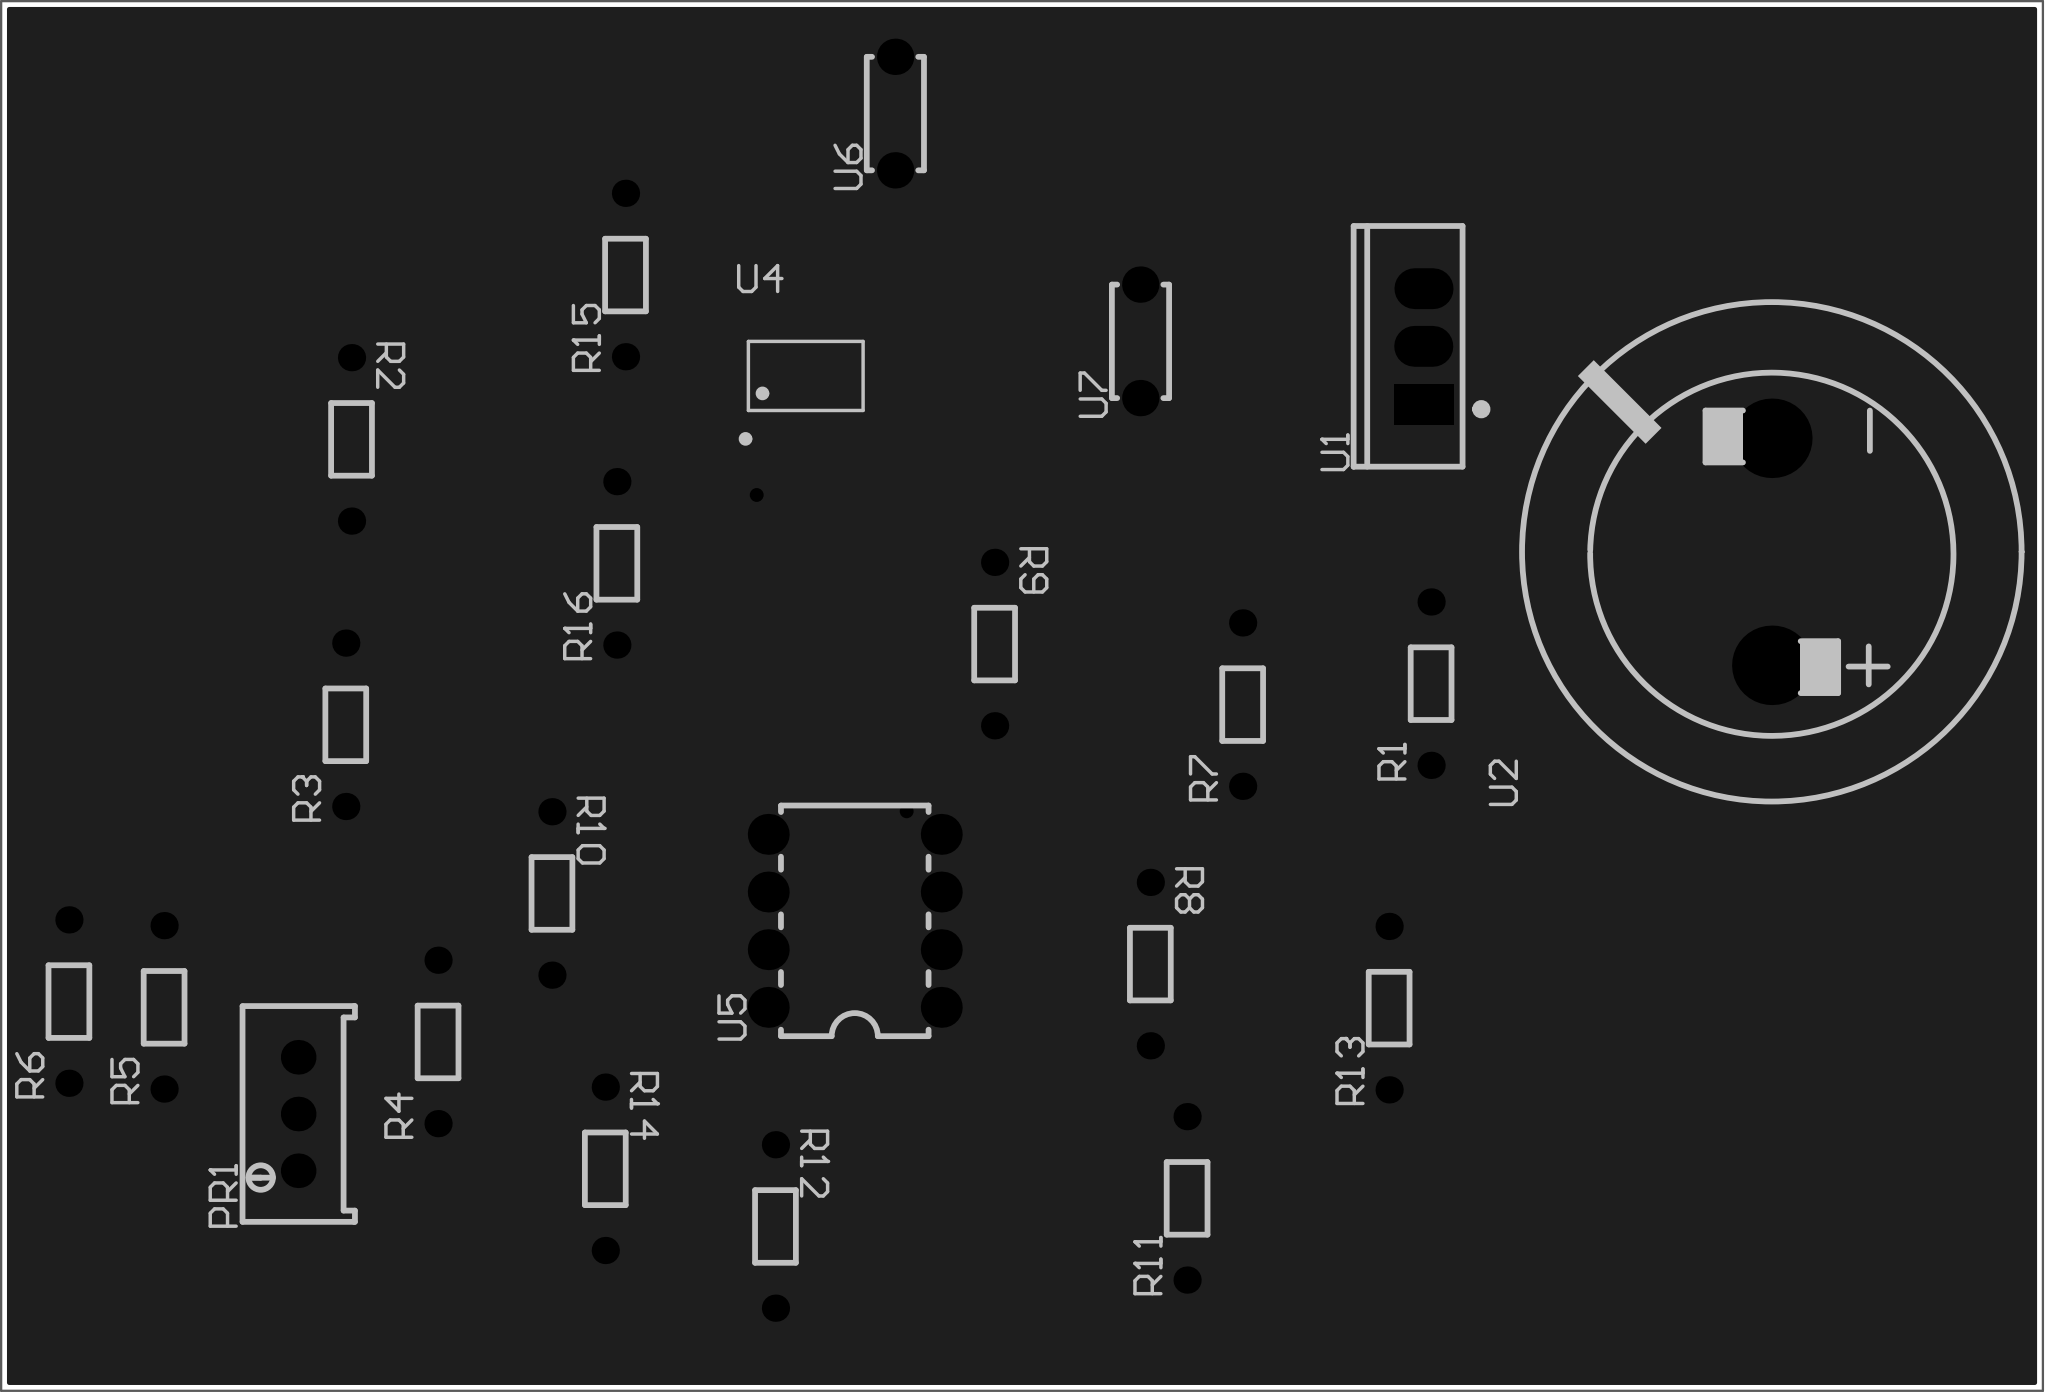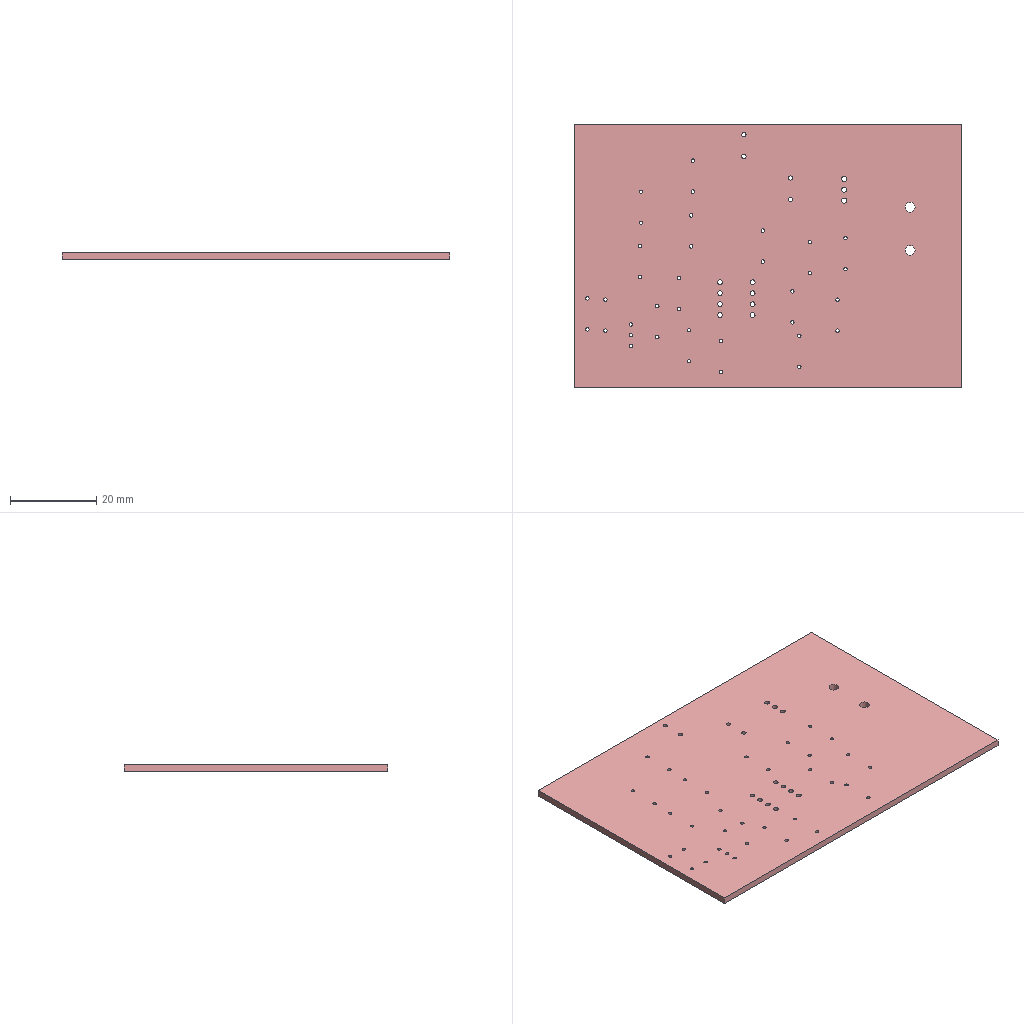Circuit board layout | Altium Designer | box 89.9 x 61.2 x 1.6 mm
Layer stack:
# Altium Designer layer stack of  (unit mm; dielectric type: 0 none, 1 core, 2 prepreg, 3 surface material)
index,name,kind,layer,copper_thickness_mm,dielectric_type,dielectric_thickness_mm,dielectric_material,dielectric_constant
0,Top Paste Mask Layer,other,,,,,,
1,Top Silkscreen Layer,other,,,,,,
2,Top Solder Mask Layer,dielectric,,,3,0.01,,3.3
3,Top Layer,copper,Top Layer,0.035,,,,
4,Dielectric1,dielectric,,,3,1.51,FR4,4.5
5,Bottom Layer,copper,Bottom Layer,0.035,,,,
6,Bottom Solder Mask Layer,dielectric,,,3,0.01,,3.3
7,Bottom Silkscreen Layer,other,,,,,,
8,Bottom Paste Mask Layer,other,,,,,,
# drill layer pairs: low layer,high layer
drill_pair,Top Layer,Bottom Layer
Part placement:
Designator,Comment,Layer,Footprint,Center-X(mm),Center-Y(mm),Rotation
PR1,10kΩ,TopLayer,R_3296,102.362,94.234,90
R1,1kΩ,TopLayer,Res_1/8W,152.254,113.191,90
R2,1.1kΩ,TopLayer,Res_1/8W,104.711,123.952,270
R3,1.1kΩ,TopLayer,Res_1/8W,104.458,111.379,90
R4,1Ω,TopLayer,Res_1/8W,108.522,97.409,90
R5,1Ω,TopLayer,Res_1/8W,96.457,98.933,90
R6,1Ω,TopLayer,Res_1/8W,92.266,99.187,90
R7,1.1kΩ,TopLayer,Res_1/8W,143.955,112.268,90
R8,500Ω,TopLayer,Res_1/8W,139.89,100.838,270
R9,10kΩ,TopLayer,Res_1/8W,133.032,114.935,270
R10,400KΩ,TopLayer,Res_1/8W,113.538,103.95,270
R11,100kΩ,TopLayer,Res_1/8W,141.509,90.519,90
R12,100kΩ,TopLayer,Res_1/8W,123.381,89.281,270
R13,100kΩ,TopLayer,Res_1/8W,150.406,98.898,90
R14,100kΩ,TopLayer,Res_1/8W,115.887,91.821,270
R15,1kΩ,TopLayer,Res_1/8W,116.777,131.191,90
R16,1kΩ,TopLayer,Res_1/8W,116.396,118.491,90
U1,LM7805CT,TopLayer,TO-220-3_L10.0-W4.5-P2.54-L,151.936,128.05,90
U2,820uF,TopLayer,CAP-TH_BD22.0-P10.00-D2.2-FD,167.259,118.999,90
U4,LM358ADR-EV,TopLayer,SOIC-8_L4.9-W3.9-P1.27-LS6.0-BL,124.714,126.746,0
U5,LM358AN/NOPB,TopLayer,PDIP-8_L10.2-W6.5-P2.54-LS7.6-BL,126.873,102.743,90
U6,2.4UF,TopLayer,CAP-TH_L5.0-W2.5-P5.00-D1.0,128.651,138.303,90
U7,1.2UF,TopLayer,CAP-TH_L5.0-W2.5-P5.00-D1.0,139.446,128.27,90
Pad and via stacks:
# Altium Designer via and pad stacks of  (unit mm). Each distinct definition once, with the count of objects using it.
# via: kind,start_layer,end_layer,hole_mm,diameter_mm,mode(0 simple;1 top-mid-bottom;2 full stack),diameter_per_layer,count,example_net
# pad: kind,layer,hole_mm,hole_type(0 round;1 square;2 slot),plating,top_size,top_shape(1 round;2 rect;3 octagon;9 rounded rect),mid_size,bottom_size,mode,footprint,size_per_layer,count,example
pad,Multi-Layer,0.762,0,plated,1.524x1.524,1,1.524x1.524,1.524x1.524,0,R_3296,,3,PR1.2
pad,Multi-Layer,0.8001,0,plated,1.199x1.199,1,1.199x1.199,1.199x1.199,0,Res_1/8W,,32,R1.1
pad,Multi-Layer,1.2,0,plated,1.8x2.6,1,1.8x2.6,1.8x2.6,0,TO-220-3_L10.0-W4.5-P2.54-L,,2,U1.2
pad,Multi-Layer,1.2,0,plated,1.8x2.6,2,1.8x2.6,1.8x2.6,0,TO-220-3_L10.0-W4.5-P2.54-L,,1,U1.1
pad,Multi-Layer,2.3,0,plated,3.5x3.5,1,3.5x3.5,3.5x3.5,0,CAP-TH_BD22.0-P10.00-D2.2-FD,,2,U2.2
pad,Multi-Layer,1.1,0,plated,1.8x1.8,1,1.8x1.8,1.8x1.8,0,PDIP-8_L10.2-W6.5-P2.54-LS7.6-BL,,8,U5.1
pad,Multi-Layer,1,0,plated,1.6x1.6,1,1.6x1.6,1.6x1.6,0,CAP-TH_L5.0-W2.5-P5.00-D1.0,,4,U6.1
pad,Top Layer,0,0,plated,0.588x2.045,1,0.588x2.045,0.588x2.045,0,SOIC-8_L4.9-W3.9-P1.27-LS6.0-BL,,8,U4.5
via,Top Layer,Bottom Layer,0.3048,0.61,0,,2,UO4
Copper pours:
name,layer,net,type(0 solid;1 hatched;2 none)
Top Layer-GND,Top Layer,GND,0